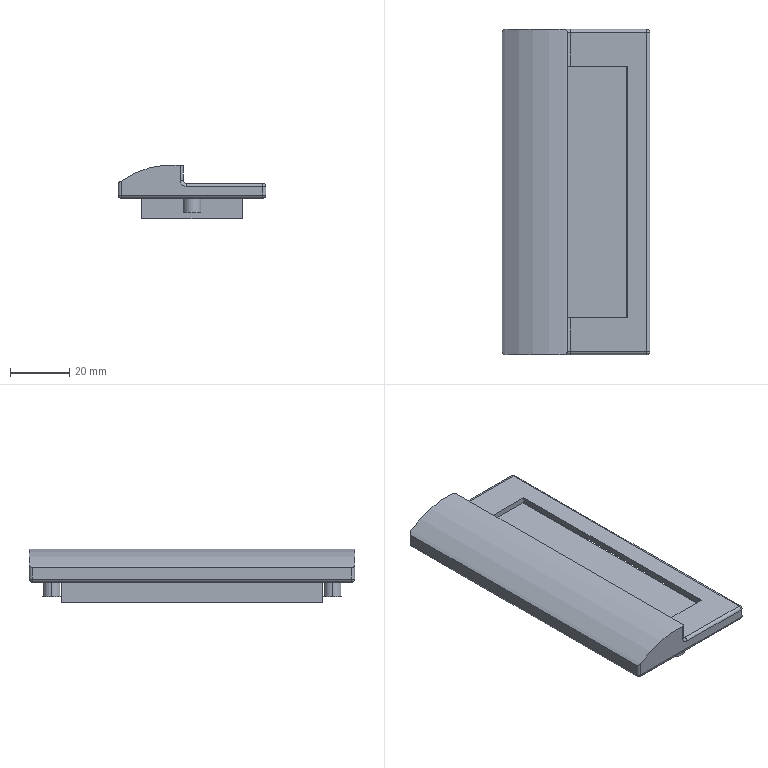Part | STEP file | Embedded H-122 | 2 solids | 59 faces | box 50 x 110 x 18.248 mm | volume 44463 mm3 | plane 27 | cylinder 24 | sphere 6 | torus 2 | commonest cylinder face diameters 2 x15 5 x4 6 x4 59.127 x1